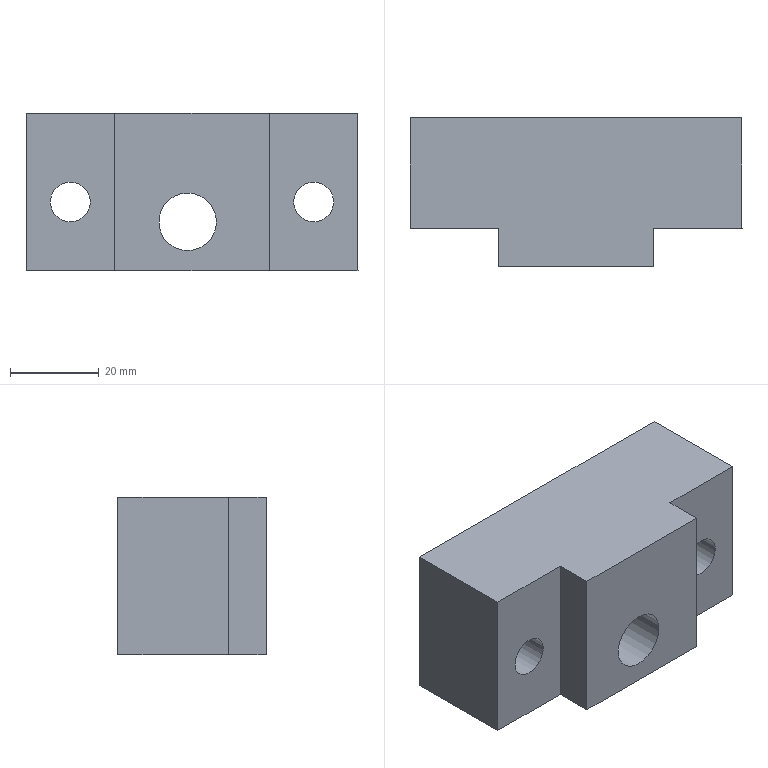Part | NX | features MAIN_BODY 2 | 1 solid | 15 faces | box 75 x 33.5 x 35.5 mm | volume 66140 mm3 | plane 11 | cylinder 4 | commonest cylinder face diameters 9 x2 13 x1 20 x1
STEP:
#1=CARTESIAN_POINT('',(-268.,138.5,359.));
#2=VERTEX_POINT('',#1);
#3=CARTESIAN_POINT('',(-268.,138.5,363.5));
#4=DIRECTION('',(0.,-1.,0.));
#5=DIRECTION('',(0.,0.,-1.));
#6=AXIS2_PLACEMENT_3D('',#3,#4,#5);
#7=CIRCLE('',#6,4.5);
#8=EDGE_CURVE('',#2,#2,#7,.F.);
#9=ORIENTED_EDGE('',*,*,#8,.F.);
#10=EDGE_LOOP('',(#9));
#11=FACE_BOUND('',#10,.T.);
#12=CARTESIAN_POINT('',(-323.,138.5,359.));
#13=VERTEX_POINT('',#12);
#14=CARTESIAN_POINT('',(-323.,138.5,363.5));
#15=DIRECTION('',(0.,-1.,0.));
#16=DIRECTION('',(0.,0.,-1.));
#17=AXIS2_PLACEMENT_3D('',#14,#15,#16);
#18=CIRCLE('',#17,4.5);
#19=EDGE_CURVE('',#13,#13,#18,.F.);
#20=ORIENTED_EDGE('',*,*,#19,.F.);
#21=EDGE_LOOP('',(#20));
#22=FACE_BOUND('',#21,.T.);
#23=CARTESIAN_POINT('',(-258.,138.5,383.5));
#24=VERTEX_POINT('',#23);
#25=CARTESIAN_POINT('',(-258.,138.5,348.));
#26=VERTEX_POINT('',#25);
#27=CARTESIAN_POINT('',(-258.,138.5,380.));
#28=DIRECTION('',(-0.000000001,0.,1.));
#29=VECTOR('',#28,1000.);
#30=LINE('',#27,#29);
#31=EDGE_CURVE('',#24,#26,#30,.F.);
#32=ORIENTED_EDGE('',*,*,#31,.T.);
#33=CARTESIAN_POINT('',(-333.,138.5,348.));
#34=VERTEX_POINT('',#33);
#35=CARTESIAN_POINT('',(-570.,138.5,348.));
#36=DIRECTION('',(-1.,0.,-0.000000001));
#37=VECTOR('',#36,1000.);
#38=LINE('',#35,#37);
#39=EDGE_CURVE('',#34,#26,#38,.F.);
#40=ORIENTED_EDGE('',*,*,#39,.F.);
#41=CARTESIAN_POINT('',(-333.,138.5,383.5));
#42=VERTEX_POINT('',#41);
#43=CARTESIAN_POINT('',(-333.,138.5,380.));
#44=DIRECTION('',(0.000000001,0.,-1.));
#45=VECTOR('',#44,1000.);
#46=LINE('',#43,#45);
#47=EDGE_CURVE('',#34,#42,#46,.F.);
#48=ORIENTED_EDGE('',*,*,#47,.T.);
#49=CARTESIAN_POINT('',(-570.,138.5,383.5));
#50=DIRECTION('',(-1.,0.,-0.000000001));
#51=VECTOR('',#50,1000.);
#52=LINE('',#49,#51);
#53=EDGE_CURVE('',#42,#24,#52,.F.);
#54=ORIENTED_EDGE('',*,*,#53,.T.);
#55=EDGE_LOOP('',(#32,#40,#48,#54));
#56=FACE_BOUND('',#55,.T.);
#57=CARTESIAN_POINT('',(-296.5,138.5,349.));
#58=VERTEX_POINT('',#57);
#59=CARTESIAN_POINT('',(-296.5,138.5,359.));
#60=DIRECTION('',(0.,-1.,0.));
#61=DIRECTION('',(0.,0.,-1.));
#62=AXIS2_PLACEMENT_3D('',#59,#60,#61);
#63=CIRCLE('',#62,10.);
#64=EDGE_CURVE('',#58,#58,#63,.F.);
#65=ORIENTED_EDGE('',*,*,#64,.F.);
#66=EDGE_LOOP('',(#65));
#67=FACE_BOUND('',#66,.T.);
#68=CARTESIAN_POINT('',(-570.,138.5,380.));
#69=DIRECTION('',(0.,-1.,0.));
#70=DIRECTION('',(0.,0.,1.));
#71=AXIS2_PLACEMENT_3D('',#68,#69,#70);
#72=PLANE('',#71);
#73=ADVANCED_FACE('',(#11,#22,#56,#67),#72,.F.);
#74=CARTESIAN_POINT('',(-296.5,105.,352.5));
#75=VERTEX_POINT('',#74);
#76=CARTESIAN_POINT('',(-296.5,105.,359.));
#77=DIRECTION('',(0.000000011,-1.,0.00000017));
#78=DIRECTION('',(0.000000001,-0.00000017,-1.));
#79=AXIS2_PLACEMENT_3D('',#76,#77,#78);
#80=CIRCLE('',#79,6.5);
#81=EDGE_CURVE('',#75,#75,#80,.T.);
#82=ORIENTED_EDGE('',*,*,#81,.T.);
#83=EDGE_LOOP('',(#82));
#84=FACE_BOUND('',#83,.T.);
#85=CARTESIAN_POINT('',(-296.5,120.,365.5));
#86=VERTEX_POINT('',#85);
#87=CARTESIAN_POINT('',(-296.5,120.,359.));
#88=DIRECTION('',(-0.000000011,1.,-0.00000017));
#89=DIRECTION('',(0.,0.00000017,1.));
#90=AXIS2_PLACEMENT_3D('',#87,#88,#89);
#91=CIRCLE('',#90,6.5);
#92=EDGE_CURVE('',#86,#86,#91,.T.);
#93=ORIENTED_EDGE('',*,*,#92,.T.);
#94=EDGE_LOOP('',(#93));
#95=FACE_BOUND('',#94,.T.);
#96=CARTESIAN_POINT('',(-296.5,131.,359.));
#97=DIRECTION('',(0.000000011,-1.,0.00000017));
#98=DIRECTION('',(-0.000000001,0.00000017,1.));
#99=AXIS2_PLACEMENT_3D('',#96,#97,#98);
#100=CYLINDRICAL_SURFACE('',#99,6.5);
#101=ADVANCED_FACE('',(#84,#95),#100,.F.);
#102=CARTESIAN_POINT('',(-323.,113.5,368.));
#103=VERTEX_POINT('',#102);
#104=CARTESIAN_POINT('',(-323.,113.5,363.5));
#105=DIRECTION('',(-0.000000011,1.,-0.00000017));
#106=DIRECTION('',(0.,0.00000017,1.));
#107=AXIS2_PLACEMENT_3D('',#104,#105,#106);
#108=CIRCLE('',#107,4.5);
#109=EDGE_CURVE('',#103,#103,#108,.T.);
#110=ORIENTED_EDGE('',*,*,#109,.T.);
#111=EDGE_LOOP('',(#110));
#112=FACE_BOUND('',#111,.T.);
#113=CARTESIAN_POINT('',(-313.,113.5,383.5));
#114=VERTEX_POINT('',#113);
#115=CARTESIAN_POINT('',(-313.,113.5,348.));
#116=VERTEX_POINT('',#115);
#117=CARTESIAN_POINT('',(-313.,113.5,361.));
#118=DIRECTION('',(-0.000000001,0.00000017,1.));
#119=VECTOR('',#118,1000.);
#120=LINE('',#117,#119);
#121=EDGE_CURVE('',#114,#116,#120,.F.);
#122=ORIENTED_EDGE('',*,*,#121,.F.);
#123=CARTESIAN_POINT('',(-333.,113.5,383.5));
#124=VERTEX_POINT('',#123);
#125=CARTESIAN_POINT('',(-313.,113.5,383.5));
#126=DIRECTION('',(1.,0.000000011,0.000000001));
#127=VECTOR('',#126,1000.);
#128=LINE('',#125,#127);
#129=EDGE_CURVE('',#124,#114,#128,.T.);
#130=ORIENTED_EDGE('',*,*,#129,.F.);
#131=CARTESIAN_POINT('',(-333.,113.5,348.));
#132=VERTEX_POINT('',#131);
#133=CARTESIAN_POINT('',(-333.,113.5,361.));
#134=DIRECTION('',(-0.000000001,0.00000017,1.));
#135=VECTOR('',#134,1000.);
#136=LINE('',#133,#135);
#137=EDGE_CURVE('',#132,#124,#136,.T.);
#138=ORIENTED_EDGE('',*,*,#137,.F.);
#139=CARTESIAN_POINT('',(-313.,113.5,348.));
#140=DIRECTION('',(1.,0.000000011,0.000000001));
#141=VECTOR('',#140,1000.);
#142=LINE('',#139,#141);
#143=EDGE_CURVE('',#132,#116,#142,.T.);
#144=ORIENTED_EDGE('',*,*,#143,.T.);
#145=EDGE_LOOP('',(#122,#130,#138,#144));
#146=FACE_BOUND('',#145,.T.);
#147=CARTESIAN_POINT('',(-313.,113.5,361.));
#148=DIRECTION('',(-0.000000011,1.,-0.00000017));
#149=DIRECTION('',(0.000000001,-0.00000017,-1.));
#150=AXIS2_PLACEMENT_3D('',#147,#148,#149);
#151=PLANE('',#150);
#152=ADVANCED_FACE('',(#112,#146),#151,.F.);
#153=CARTESIAN_POINT('',(-268.,113.5,368.));
#154=VERTEX_POINT('',#153);
#155=CARTESIAN_POINT('',(-268.,113.5,363.5));
#156=DIRECTION('',(-0.000000011,1.,-0.00000017));
#157=DIRECTION('',(0.,0.00000017,1.));
#158=AXIS2_PLACEMENT_3D('',#155,#156,#157);
#159=CIRCLE('',#158,4.5);
#160=EDGE_CURVE('',#154,#154,#159,.T.);
#161=ORIENTED_EDGE('',*,*,#160,.T.);
#162=EDGE_LOOP('',(#161));
#163=FACE_BOUND('',#162,.T.);
#164=CARTESIAN_POINT('',(-278.,113.5,348.));
#165=VERTEX_POINT('',#164);
#166=CARTESIAN_POINT('',(-278.,113.5,383.5));
#167=VERTEX_POINT('',#166);
#168=CARTESIAN_POINT('',(-278.,113.5,361.));
#169=DIRECTION('',(-0.000000001,0.00000017,1.));
#170=VECTOR('',#169,1000.);
#171=LINE('',#168,#170);
#172=EDGE_CURVE('',#165,#167,#171,.T.);
#173=ORIENTED_EDGE('',*,*,#172,.F.);
#174=CARTESIAN_POINT('',(-258.,113.5,348.));
#175=VERTEX_POINT('',#174);
#176=CARTESIAN_POINT('',(-313.,113.5,348.));
#177=DIRECTION('',(1.,0.000000011,0.000000001));
#178=VECTOR('',#177,1000.);
#179=LINE('',#176,#178);
#180=EDGE_CURVE('',#165,#175,#179,.T.);
#181=ORIENTED_EDGE('',*,*,#180,.T.);
#182=CARTESIAN_POINT('',(-258.,113.5,383.5));
#183=VERTEX_POINT('',#182);
#184=CARTESIAN_POINT('',(-258.,113.5,361.));
#185=DIRECTION('',(0.000000001,-0.00000017,-1.));
#186=VECTOR('',#185,1000.);
#187=LINE('',#184,#186);
#188=EDGE_CURVE('',#183,#175,#187,.T.);
#189=ORIENTED_EDGE('',*,*,#188,.F.);
#190=CARTESIAN_POINT('',(-313.,113.5,383.5));
#191=DIRECTION('',(1.,0.000000011,0.000000001));
#192=VECTOR('',#191,1000.);
#193=LINE('',#190,#192);
#194=EDGE_CURVE('',#167,#183,#193,.T.);
#195=ORIENTED_EDGE('',*,*,#194,.F.);
#196=EDGE_LOOP('',(#173,#181,#189,#195));
#197=FACE_BOUND('',#196,.T.);
#198=CARTESIAN_POINT('',(-313.,113.5,361.));
#199=DIRECTION('',(-0.000000011,1.,-0.00000017));
#200=DIRECTION('',(0.000000001,-0.00000017,-1.));
#201=AXIS2_PLACEMENT_3D('',#198,#199,#200);
#202=PLANE('',#201);
#203=ADVANCED_FACE('',(#163,#197),#202,.F.);
#204=CARTESIAN_POINT('',(-278.,105.,383.5));
#205=VERTEX_POINT('',#204);
#206=CARTESIAN_POINT('',(-278.,125.,383.5));
#207=DIRECTION('',(0.000000011,-1.,0.00000017));
#208=VECTOR('',#207,1000.);
#209=LINE('',#206,#208);
#210=EDGE_CURVE('',#205,#167,#209,.F.);
#211=ORIENTED_EDGE('',*,*,#210,.T.);
#212=ORIENTED_EDGE('',*,*,#194,.T.);
#213=CARTESIAN_POINT('',(-258.,125.,383.5));
#214=DIRECTION('',(-0.000000011,1.,-0.00000017));
#215=VECTOR('',#214,1000.);
#216=LINE('',#213,#215);
#217=EDGE_CURVE('',#183,#24,#216,.T.);
#218=ORIENTED_EDGE('',*,*,#217,.T.);
#219=ORIENTED_EDGE('',*,*,#53,.F.);
#220=CARTESIAN_POINT('',(-333.,125.,383.5));
#221=DIRECTION('',(-0.000000011,1.,-0.00000017));
#222=VECTOR('',#221,1000.);
#223=LINE('',#220,#222);
#224=EDGE_CURVE('',#124,#42,#223,.T.);
#225=ORIENTED_EDGE('',*,*,#224,.F.);
#226=ORIENTED_EDGE('',*,*,#129,.T.);
#227=CARTESIAN_POINT('',(-313.,105.,383.5));
#228=VERTEX_POINT('',#227);
#229=CARTESIAN_POINT('',(-313.,125.,383.5));
#230=DIRECTION('',(-0.000000011,1.,-0.00000017));
#231=VECTOR('',#230,1000.);
#232=LINE('',#229,#231);
#233=EDGE_CURVE('',#228,#114,#232,.T.);
#234=ORIENTED_EDGE('',*,*,#233,.F.);
#235=CARTESIAN_POINT('',(-376.5,105.,383.5));
#236=DIRECTION('',(1.,0.000000011,0.000000001));
#237=VECTOR('',#236,1000.);
#238=LINE('',#235,#237);
#239=EDGE_CURVE('',#228,#205,#238,.T.);
#240=ORIENTED_EDGE('',*,*,#239,.T.);
#241=EDGE_LOOP('',(#211,#212,#218,#219,#225,#226,#234,#240));
#242=FACE_BOUND('',#241,.T.);
#243=CARTESIAN_POINT('',(-376.5,125.,383.5));
#244=DIRECTION('',(-0.000000001,0.00000017,1.));
#245=DIRECTION('',(1.,0.000000011,0.000000001));
#246=AXIS2_PLACEMENT_3D('',#243,#244,#245);
#247=PLANE('',#246);
#248=ADVANCED_FACE('',(#242),#247,.T.);
#249=ORIENTED_EDGE('',*,*,#47,.F.);
#250=CARTESIAN_POINT('',(-333.,125.,348.));
#251=DIRECTION('',(-0.000000011,1.,-0.00000017));
#252=VECTOR('',#251,1000.);
#253=LINE('',#250,#252);
#254=EDGE_CURVE('',#132,#34,#253,.T.);
#255=ORIENTED_EDGE('',*,*,#254,.F.);
#256=ORIENTED_EDGE('',*,*,#137,.T.);
#257=ORIENTED_EDGE('',*,*,#224,.T.);
#258=EDGE_LOOP('',(#249,#255,#256,#257));
#259=FACE_BOUND('',#258,.T.);
#260=CARTESIAN_POINT('',(-333.,125.,361.));
#261=DIRECTION('',(-1.,-0.000000011,-0.000000001));
#262=DIRECTION('',(-0.000000001,0.00000017,1.));
#263=AXIS2_PLACEMENT_3D('',#260,#261,#262);
#264=PLANE('',#263);
#265=ADVANCED_FACE('',(#259),#264,.T.);
#266=ORIENTED_EDGE('',*,*,#180,.F.);
#267=CARTESIAN_POINT('',(-278.,105.,348.));
#268=VERTEX_POINT('',#267);
#269=CARTESIAN_POINT('',(-278.,125.,348.));
#270=DIRECTION('',(-0.000000011,1.,-0.00000017));
#271=VECTOR('',#270,1000.);
#272=LINE('',#269,#271);
#273=EDGE_CURVE('',#268,#165,#272,.T.);
#274=ORIENTED_EDGE('',*,*,#273,.F.);
#275=CARTESIAN_POINT('',(-313.,105.,348.));
#276=VERTEX_POINT('',#275);
#277=CARTESIAN_POINT('',(-313.,105.,348.));
#278=DIRECTION('',(1.,0.000000011,0.000000001));
#279=VECTOR('',#278,1000.);
#280=LINE('',#277,#279);
#281=EDGE_CURVE('',#276,#268,#280,.T.);
#282=ORIENTED_EDGE('',*,*,#281,.F.);
#283=CARTESIAN_POINT('',(-313.,146.,348.));
#284=DIRECTION('',(0.000000011,-1.,0.00000017));
#285=VECTOR('',#284,1000.);
#286=LINE('',#283,#285);
#287=EDGE_CURVE('',#276,#116,#286,.F.);
#288=ORIENTED_EDGE('',*,*,#287,.T.);
#289=ORIENTED_EDGE('',*,*,#143,.F.);
#290=ORIENTED_EDGE('',*,*,#254,.T.);
#291=ORIENTED_EDGE('',*,*,#39,.T.);
#292=CARTESIAN_POINT('',(-258.,146.,348.));
#293=DIRECTION('',(-0.000000011,1.,-0.00000017));
#294=VECTOR('',#293,1000.);
#295=LINE('',#292,#294);
#296=EDGE_CURVE('',#175,#26,#295,.T.);
#297=ORIENTED_EDGE('',*,*,#296,.F.);
#298=EDGE_LOOP('',(#266,#274,#282,#288,#289,#290,#291,#297));
#299=FACE_BOUND('',#298,.T.);
#300=CARTESIAN_POINT('',(-188.,146.,348.));
#301=DIRECTION('',(-0.000000001,0.00000017,1.));
#302=DIRECTION('',(1.,0.000000011,0.000000001));
#303=AXIS2_PLACEMENT_3D('',#300,#301,#302);
#304=PLANE('',#303);
#305=ADVANCED_FACE('',(#299),#304,.F.);
#306=ORIENTED_EDGE('',*,*,#31,.F.);
#307=ORIENTED_EDGE('',*,*,#217,.F.);
#308=ORIENTED_EDGE('',*,*,#188,.T.);
#309=ORIENTED_EDGE('',*,*,#296,.T.);
#310=EDGE_LOOP('',(#306,#307,#308,#309));
#311=FACE_BOUND('',#310,.T.);
#312=CARTESIAN_POINT('',(-258.,125.,361.));
#313=DIRECTION('',(1.,0.000000011,0.000000001));
#314=DIRECTION('',(0.000000001,-0.00000017,-1.));
#315=AXIS2_PLACEMENT_3D('',#312,#313,#314);
#316=PLANE('',#315);
#317=ADVANCED_FACE('',(#311),#316,.T.);
#318=ORIENTED_EDGE('',*,*,#233,.T.);
#319=ORIENTED_EDGE('',*,*,#121,.T.);
#320=ORIENTED_EDGE('',*,*,#287,.F.);
#321=CARTESIAN_POINT('',(-313.,105.,358.5));
#322=DIRECTION('',(0.000000001,-0.00000017,-1.));
#323=VECTOR('',#322,1000.);
#324=LINE('',#321,#323);
#325=EDGE_CURVE('',#276,#228,#324,.F.);
#326=ORIENTED_EDGE('',*,*,#325,.T.);
#327=EDGE_LOOP('',(#318,#319,#320,#326));
#328=FACE_BOUND('',#327,.T.);
#329=CARTESIAN_POINT('',(-313.,125.,358.5));
#330=DIRECTION('',(-1.,-0.000000011,-0.000000001));
#331=DIRECTION('',(-0.000000001,0.00000017,1.));
#332=AXIS2_PLACEMENT_3D('',#329,#330,#331);
#333=PLANE('',#332);
#334=ADVANCED_FACE('',(#328),#333,.T.);
#335=ORIENTED_EDGE('',*,*,#273,.T.);
#336=ORIENTED_EDGE('',*,*,#172,.T.);
#337=ORIENTED_EDGE('',*,*,#210,.F.);
#338=CARTESIAN_POINT('',(-278.,105.,358.5));
#339=DIRECTION('',(-0.000000001,0.00000017,1.));
#340=VECTOR('',#339,1000.);
#341=LINE('',#338,#340);
#342=EDGE_CURVE('',#268,#205,#341,.T.);
#343=ORIENTED_EDGE('',*,*,#342,.F.);
#344=EDGE_LOOP('',(#335,#336,#337,#343));
#345=FACE_BOUND('',#344,.T.);
#346=CARTESIAN_POINT('',(-278.,125.,358.5));
#347=DIRECTION('',(-1.,-0.000000011,-0.000000001));
#348=DIRECTION('',(-0.000000001,0.00000017,1.));
#349=AXIS2_PLACEMENT_3D('',#346,#347,#348);
#350=PLANE('',#349);
#351=ADVANCED_FACE('',(#345),#350,.F.);
#352=ORIENTED_EDGE('',*,*,#81,.F.);
#353=EDGE_LOOP('',(#352));
#354=FACE_BOUND('',#353,.T.);
#355=ORIENTED_EDGE('',*,*,#342,.T.);
#356=ORIENTED_EDGE('',*,*,#239,.F.);
#357=ORIENTED_EDGE('',*,*,#325,.F.);
#358=ORIENTED_EDGE('',*,*,#281,.T.);
#359=EDGE_LOOP('',(#355,#356,#357,#358));
#360=FACE_BOUND('',#359,.T.);
#361=CARTESIAN_POINT('',(-313.,105.,358.5));
#362=DIRECTION('',(-0.000000011,1.,-0.00000017));
#363=DIRECTION('',(0.000000001,-0.00000017,-1.));
#364=AXIS2_PLACEMENT_3D('',#361,#362,#363);
#365=PLANE('',#364);
#366=ADVANCED_FACE('',(#354,#360),#365,.F.);
#367=ORIENTED_EDGE('',*,*,#19,.T.);
#368=EDGE_LOOP('',(#367));
#369=FACE_BOUND('',#368,.T.);
#370=ORIENTED_EDGE('',*,*,#109,.F.);
#371=EDGE_LOOP('',(#370));
#372=FACE_BOUND('',#371,.T.);
#373=CARTESIAN_POINT('',(-323.,125.,363.5));
#374=DIRECTION('',(-0.000000011,1.,-0.00000017));
#375=DIRECTION('',(-0.000000001,0.00000017,1.));
#376=AXIS2_PLACEMENT_3D('',#373,#374,#375);
#377=CYLINDRICAL_SURFACE('',#376,4.5);
#378=ADVANCED_FACE('',(#369,#372),#377,.F.);
#379=ORIENTED_EDGE('',*,*,#8,.T.);
#380=EDGE_LOOP('',(#379));
#381=FACE_BOUND('',#380,.T.);
#382=ORIENTED_EDGE('',*,*,#160,.F.);
#383=EDGE_LOOP('',(#382));
#384=FACE_BOUND('',#383,.T.);
#385=CARTESIAN_POINT('',(-268.,125.,363.5));
#386=DIRECTION('',(-0.000000011,1.,-0.00000017));
#387=DIRECTION('',(-0.000000001,0.00000017,1.));
#388=AXIS2_PLACEMENT_3D('',#385,#386,#387);
#389=CYLINDRICAL_SURFACE('',#388,4.5);
#390=ADVANCED_FACE('',(#381,#384),#389,.F.);
#391=CARTESIAN_POINT('',(-296.5,120.,369.));
#392=VERTEX_POINT('',#391);
#393=CARTESIAN_POINT('',(-296.5,120.,359.));
#394=DIRECTION('',(-0.000000011,1.,-0.00000017));
#395=DIRECTION('',(0.,0.00000017,1.));
#396=AXIS2_PLACEMENT_3D('',#393,#394,#395);
#397=CIRCLE('',#396,10.);
#398=EDGE_CURVE('',#392,#392,#397,.F.);
#399=ORIENTED_EDGE('',*,*,#398,.F.);
#400=EDGE_LOOP('',(#399));
#401=FACE_BOUND('',#400,.T.);
#402=ORIENTED_EDGE('',*,*,#92,.F.);
#403=EDGE_LOOP('',(#402));
#404=FACE_BOUND('',#403,.T.);
#405=CARTESIAN_POINT('',(-296.5,120.,359.));
#406=DIRECTION('',(-0.000000011,1.,-0.00000017));
#407=DIRECTION('',(0.000000001,-0.00000017,-1.));
#408=AXIS2_PLACEMENT_3D('',#405,#406,#407);
#409=PLANE('',#408);
#410=ADVANCED_FACE('',(#401,#404),#409,.T.);
#411=ORIENTED_EDGE('',*,*,#64,.T.);
#412=EDGE_LOOP('',(#411));
#413=FACE_BOUND('',#412,.T.);
#414=ORIENTED_EDGE('',*,*,#398,.T.);
#415=EDGE_LOOP('',(#414));
#416=FACE_BOUND('',#415,.T.);
#417=CARTESIAN_POINT('',(-296.5,131.,359.));
#418=DIRECTION('',(0.000000011,-1.,0.00000017));
#419=DIRECTION('',(-0.000000001,0.00000017,1.));
#420=AXIS2_PLACEMENT_3D('',#417,#418,#419);
#421=CYLINDRICAL_SURFACE('',#420,10.);
#422=ADVANCED_FACE('',(#413,#416),#421,.F.);
#423=CLOSED_SHELL('',(#73,#101,#152,#203,#248,#265,#305,#317,#334,#351,#366,#378,#390,#410,#422));
#424=MANIFOLD_SOLID_BREP('',#423);
#425=(LENGTH_UNIT()NAMED_UNIT(*)SI_UNIT(.MILLI.,.METRE.));
#426=UNCERTAINTY_MEASURE_WITH_UNIT(LENGTH_MEASURE(0.00001),#425,'','');
#427=(NAMED_UNIT(*)PLANE_ANGLE_UNIT()SI_UNIT($,.RADIAN.));
#428=(NAMED_UNIT(*)SI_UNIT($,.STERADIAN.)SOLID_ANGLE_UNIT());
#429=(GEOMETRIC_REPRESENTATION_CONTEXT(3)GLOBAL_UNCERTAINTY_ASSIGNED_CONTEXT((#426))GLOBAL_UNIT_ASSIGNED_CONTEXT((#425,#427,#428))REPRESENTATION_CONTEXT('',''));
#430=ADVANCED_BREP_SHAPE_REPRESENTATION('',(#424),#429);